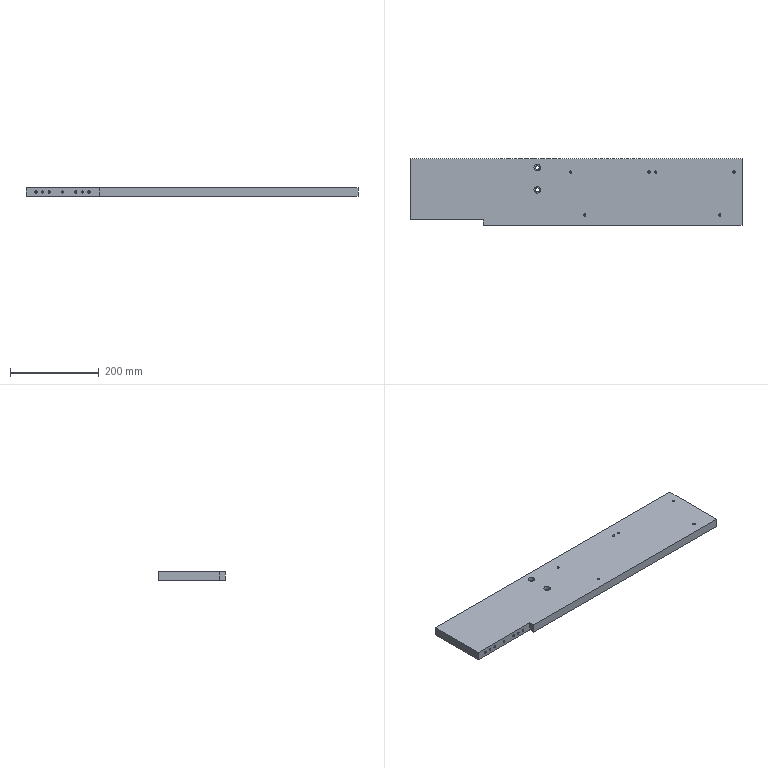Part | NX | features BREP 1 | 1 solid | 78 faces | box 750 x 150 x 20 mm | volume 2199299 mm3 | cylinder 46 | cone 18 | plane 14 | commonest cylinder face diameters 5 x30 6.8 x8 9 x4 15 x4